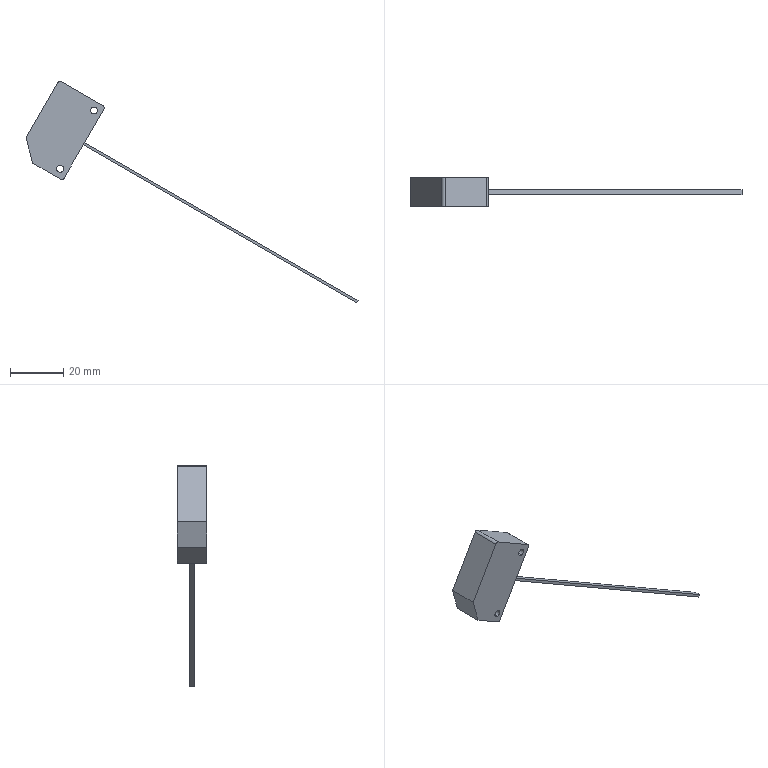Part | STEP file | optexzd-l40n | 1 solid | 29 faces | box 125.041 x 11 x 83.373 mm | volume 6875 mm3 | plane 19 | cylinder 10 | commonest cylinder face diameters 2 x4 2.6 x4 1 x2